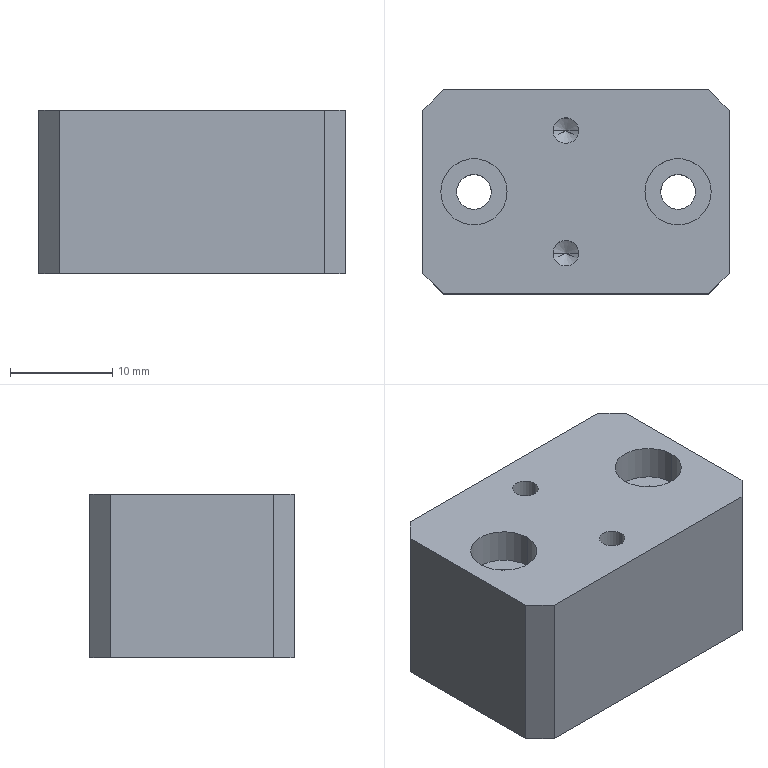Part | STEP file | QA-AD21 | 1 solid | 28 faces | box 30 x 20 x 16 mm | volume 8932 mm3 | cylinder 12 | plane 12 | cone 4 | commonest cylinder face diameters 2.5 x4 3.4 x4 6.5 x4